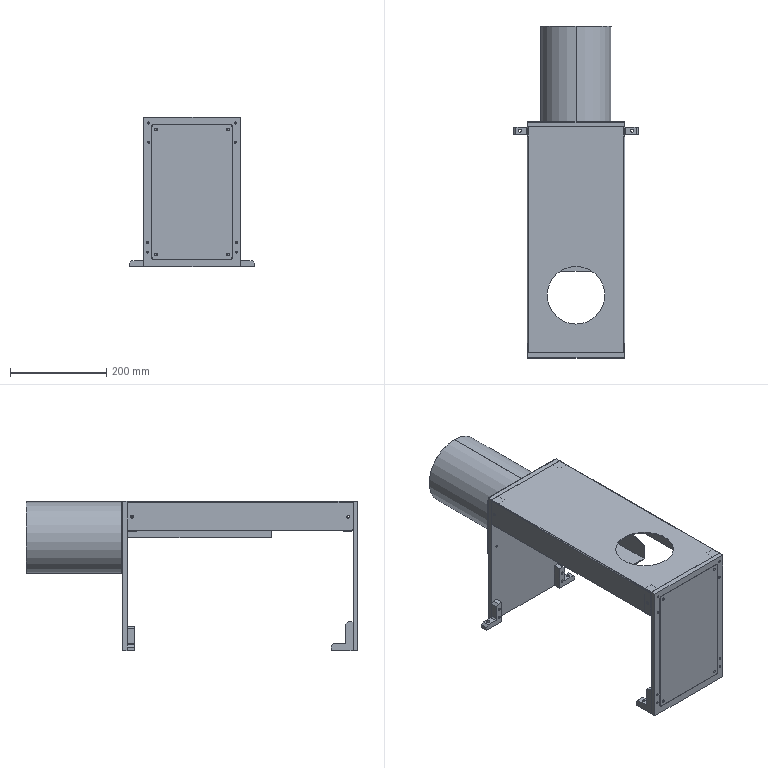Part | SolidWorks | 14 solids | 333 faces | box 260 x 690 x 310 mm | volume 1689497 mm3 | cylinder 180 | plane 153 | commonest cylinder face diameters 4.2 x60 5.5 x44 10 x24 6 x22 6.5 x8 20 x8